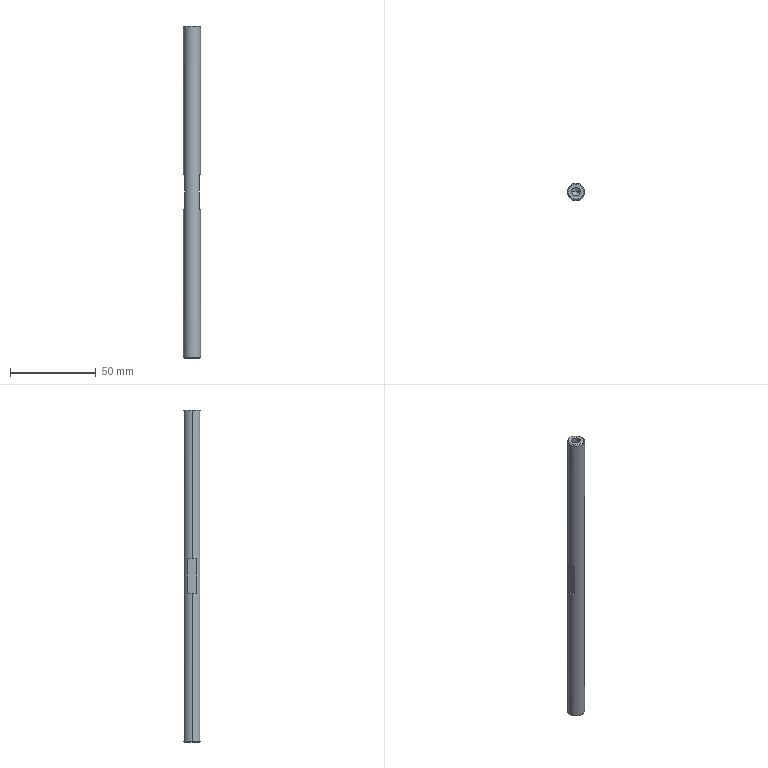Part | SolidWorks | features HoleWzd 2, Chamfer 1, Extrusion 1, ICE 1 | 1 solid | 22 faces | box 10 x 10 x 194 mm | volume 14513 mm3 | cone 8 | plane 8 | cylinder 6 | commonest cylinder face diameters 5 x4 10 x2
STEP:
#1=CARTESIAN_POINT('',(-4.5,0.,-97.));
#2=VERTEX_POINT('',#1);
#3=CARTESIAN_POINT('',(4.5,0.,-97.));
#4=VERTEX_POINT('',#3);
#5=CARTESIAN_POINT('',(0.,0.,-97.));
#6=DIRECTION('',(0.,0.,-1.));
#7=DIRECTION('',(1.,0.,0.));
#8=AXIS2_PLACEMENT_3D('',#5,#6,#7);
#9=CIRCLE('',#8,4.5);
#10=EDGE_CURVE('',#2,#4,#9,.T.);
#11=ORIENTED_EDGE('',*,*,#10,.F.);
#12=CARTESIAN_POINT('',(-5.,0.,-96.5));
#13=VERTEX_POINT('',#12);
#14=CARTESIAN_POINT('',(-5.,0.,-96.5));
#15=DIRECTION('',(-0.7071,0.,0.7071));
#16=VECTOR('',#15,1000.);
#17=LINE('',#14,#16);
#18=EDGE_CURVE('',#2,#13,#17,.T.);
#19=ORIENTED_EDGE('',*,*,#18,.T.);
#20=CARTESIAN_POINT('',(5.,0.,-96.5));
#21=VERTEX_POINT('',#20);
#22=CARTESIAN_POINT('',(0.,0.,-96.5));
#23=DIRECTION('',(0.,0.,1.));
#24=DIRECTION('',(1.,0.,0.));
#25=AXIS2_PLACEMENT_3D('',#22,#23,#24);
#26=CIRCLE('',#25,5.);
#27=EDGE_CURVE('',#21,#13,#26,.T.);
#28=ORIENTED_EDGE('',*,*,#27,.F.);
#29=CARTESIAN_POINT('',(5.,0.,-96.5));
#30=DIRECTION('',(0.7071,0.,0.7071));
#31=VECTOR('',#30,1000.);
#32=LINE('',#29,#31);
#33=EDGE_CURVE('',#4,#21,#32,.T.);
#34=ORIENTED_EDGE('',*,*,#33,.F.);
#35=EDGE_LOOP('',(#11,#19,#28,#34));
#36=FACE_OUTER_BOUND('',#35,.T.);
#37=CARTESIAN_POINT('',(0.,0.,-96.5));
#38=DIRECTION('',(0.,0.,1.));
#39=DIRECTION('',(1.,0.,0.));
#40=AXIS2_PLACEMENT_3D('',#37,#38,#39);
#41=CONICAL_SURFACE('',#40,5.,0.7854);
#42=ADVANCED_FACE('',(#36),#41,.T.);
#43=CARTESIAN_POINT('',(4.5,0.,97.));
#44=VERTEX_POINT('',#43);
#45=CARTESIAN_POINT('',(-4.5,0.,97.));
#46=VERTEX_POINT('',#45);
#47=CARTESIAN_POINT('',(0.,0.,97.));
#48=DIRECTION('',(0.,0.,1.));
#49=DIRECTION('',(1.,0.,0.));
#50=AXIS2_PLACEMENT_3D('',#47,#48,#49);
#51=CIRCLE('',#50,4.5);
#52=EDGE_CURVE('',#44,#46,#51,.T.);
#53=ORIENTED_EDGE('',*,*,#52,.F.);
#54=CARTESIAN_POINT('',(5.,0.,96.5));
#55=VERTEX_POINT('',#54);
#56=CARTESIAN_POINT('',(4.5,0.,97.));
#57=DIRECTION('',(0.7071,0.,-0.7071));
#58=VECTOR('',#57,1000.);
#59=LINE('',#56,#58);
#60=EDGE_CURVE('',#44,#55,#59,.T.);
#61=ORIENTED_EDGE('',*,*,#60,.T.);
#62=CARTESIAN_POINT('',(-5.,0.,96.5));
#63=VERTEX_POINT('',#62);
#64=CARTESIAN_POINT('',(0.,0.,96.5));
#65=DIRECTION('',(0.,0.,-1.));
#66=DIRECTION('',(1.,0.,0.));
#67=AXIS2_PLACEMENT_3D('',#64,#65,#66);
#68=CIRCLE('',#67,5.);
#69=EDGE_CURVE('',#63,#55,#68,.T.);
#70=ORIENTED_EDGE('',*,*,#69,.F.);
#71=CARTESIAN_POINT('',(-4.5,0.,97.));
#72=DIRECTION('',(-0.7071,0.,-0.7071));
#73=VECTOR('',#72,1000.);
#74=LINE('',#71,#73);
#75=EDGE_CURVE('',#46,#63,#74,.T.);
#76=ORIENTED_EDGE('',*,*,#75,.F.);
#77=EDGE_LOOP('',(#53,#61,#70,#76));
#78=FACE_OUTER_BOUND('',#77,.T.);
#79=CARTESIAN_POINT('',(0.,0.,97.));
#80=DIRECTION('',(0.,0.,-1.));
#81=DIRECTION('',(-1.,0.,0.));
#82=AXIS2_PLACEMENT_3D('',#79,#80,#81);
#83=CONICAL_SURFACE('',#82,4.5,0.7854);
#84=ADVANCED_FACE('',(#78),#83,.T.);
#85=CARTESIAN_POINT('',(2.5,0.,-82.));
#86=VERTEX_POINT('',#85);
#87=CARTESIAN_POINT('',(-2.5,0.,-82.));
#88=VERTEX_POINT('',#87);
#89=CARTESIAN_POINT('',(0.,0.,-82.));
#90=DIRECTION('',(0.,0.,-1.));
#91=DIRECTION('',(-1.,0.,0.));
#92=AXIS2_PLACEMENT_3D('',#89,#90,#91);
#93=CIRCLE('',#92,2.5);
#94=EDGE_CURVE('',#86,#88,#93,.T.);
#95=ORIENTED_EDGE('',*,*,#94,.F.);
#96=CARTESIAN_POINT('',(2.5,0.,-97.));
#97=VERTEX_POINT('',#96);
#98=CARTESIAN_POINT('',(2.5,0.,-97.));
#99=DIRECTION('',(0.,0.,-1.));
#100=VECTOR('',#99,1000.);
#101=LINE('',#98,#100);
#102=EDGE_CURVE('',#86,#97,#101,.T.);
#103=ORIENTED_EDGE('',*,*,#102,.T.);
#104=CARTESIAN_POINT('',(-2.5,0.,-97.));
#105=VERTEX_POINT('',#104);
#106=CARTESIAN_POINT('',(0.,0.,-97.));
#107=DIRECTION('',(0.,0.,-1.));
#108=DIRECTION('',(-1.,0.,0.));
#109=AXIS2_PLACEMENT_3D('',#106,#107,#108);
#110=CIRCLE('',#109,2.5);
#111=EDGE_CURVE('',#97,#105,#110,.T.);
#112=ORIENTED_EDGE('',*,*,#111,.T.);
#113=CARTESIAN_POINT('',(-2.5,0.,-97.));
#114=DIRECTION('',(0.,0.,-1.));
#115=VECTOR('',#114,1000.);
#116=LINE('',#113,#115);
#117=EDGE_CURVE('',#88,#105,#116,.T.);
#118=ORIENTED_EDGE('',*,*,#117,.F.);
#119=EDGE_LOOP('',(#95,#103,#112,#118));
#120=FACE_OUTER_BOUND('',#119,.T.);
#121=CARTESIAN_POINT('',(0.,0.,-97.));
#122=DIRECTION('',(0.,0.,-1.));
#123=DIRECTION('',(-1.,0.,0.));
#124=AXIS2_PLACEMENT_3D('',#121,#122,#123);
#125=CYLINDRICAL_SURFACE('',#124,2.5);
#126=ADVANCED_FACE('',(#120),#125,.F.);
#127=CARTESIAN_POINT('',(0.,0.,-80.498));
#128=VERTEX_POINT('',#127);
#129=CARTESIAN_POINT('',(-2.5,0.,-82.));
#130=DIRECTION('',(-0.8572,0.,-0.515));
#131=VECTOR('',#130,1000.);
#132=LINE('',#129,#131);
#133=EDGE_CURVE('',#128,#88,#132,.T.);
#134=ORIENTED_EDGE('',*,*,#133,.F.);
#135=CARTESIAN_POINT('',(2.5,0.,-82.));
#136=DIRECTION('',(0.8572,0.,-0.515));
#137=VECTOR('',#136,1000.);
#138=LINE('',#135,#137);
#139=EDGE_CURVE('',#128,#86,#138,.T.);
#140=ORIENTED_EDGE('',*,*,#139,.T.);
#141=ORIENTED_EDGE('',*,*,#94,.T.);
#142=EDGE_LOOP('',(#134,#140,#141));
#143=FACE_OUTER_BOUND('',#142,.T.);
#144=CARTESIAN_POINT('',(0.,0.,-82.));
#145=DIRECTION('',(0.,0.,-1.));
#146=DIRECTION('',(-1.,0.,0.));
#147=AXIS2_PLACEMENT_3D('',#144,#145,#146);
#148=CONICAL_SURFACE('',#147,2.5,1.03);
#149=ADVANCED_FACE('',(#143),#148,.F.);
#150=CARTESIAN_POINT('',(-2.5,0.,82.));
#151=VERTEX_POINT('',#150);
#152=CARTESIAN_POINT('',(2.5,0.,82.));
#153=VERTEX_POINT('',#152);
#154=CARTESIAN_POINT('',(0.,0.,82.));
#155=DIRECTION('',(0.,0.,1.));
#156=DIRECTION('',(1.,0.,0.));
#157=AXIS2_PLACEMENT_3D('',#154,#155,#156);
#158=CIRCLE('',#157,2.5);
#159=EDGE_CURVE('',#151,#153,#158,.T.);
#160=ORIENTED_EDGE('',*,*,#159,.F.);
#161=CARTESIAN_POINT('',(-2.5,0.,97.));
#162=VERTEX_POINT('',#161);
#163=CARTESIAN_POINT('',(-2.5,0.,97.));
#164=DIRECTION('',(0.,0.,1.));
#165=VECTOR('',#164,1000.);
#166=LINE('',#163,#165);
#167=EDGE_CURVE('',#151,#162,#166,.T.);
#168=ORIENTED_EDGE('',*,*,#167,.T.);
#169=CARTESIAN_POINT('',(2.5,0.,97.));
#170=VERTEX_POINT('',#169);
#171=CARTESIAN_POINT('',(0.,0.,97.));
#172=DIRECTION('',(0.,0.,1.));
#173=DIRECTION('',(1.,0.,0.));
#174=AXIS2_PLACEMENT_3D('',#171,#172,#173);
#175=CIRCLE('',#174,2.5);
#176=EDGE_CURVE('',#162,#170,#175,.T.);
#177=ORIENTED_EDGE('',*,*,#176,.T.);
#178=CARTESIAN_POINT('',(2.5,0.,97.));
#179=DIRECTION('',(0.,0.,1.));
#180=VECTOR('',#179,1000.);
#181=LINE('',#178,#180);
#182=EDGE_CURVE('',#153,#170,#181,.T.);
#183=ORIENTED_EDGE('',*,*,#182,.F.);
#184=EDGE_LOOP('',(#160,#168,#177,#183));
#185=FACE_OUTER_BOUND('',#184,.T.);
#186=CARTESIAN_POINT('',(0.,0.,97.));
#187=DIRECTION('',(0.,0.,1.));
#188=DIRECTION('',(1.,0.,0.));
#189=AXIS2_PLACEMENT_3D('',#186,#187,#188);
#190=CYLINDRICAL_SURFACE('',#189,2.5);
#191=ADVANCED_FACE('',(#185),#190,.F.);
#192=CARTESIAN_POINT('',(0.,0.,80.498));
#193=VERTEX_POINT('',#192);
#194=CARTESIAN_POINT('',(2.5,0.,82.));
#195=DIRECTION('',(0.8572,0.,0.515));
#196=VECTOR('',#195,1000.);
#197=LINE('',#194,#196);
#198=EDGE_CURVE('',#193,#153,#197,.T.);
#199=ORIENTED_EDGE('',*,*,#198,.F.);
#200=CARTESIAN_POINT('',(-2.5,0.,82.));
#201=DIRECTION('',(-0.8572,0.,0.515));
#202=VECTOR('',#201,1000.);
#203=LINE('',#200,#202);
#204=EDGE_CURVE('',#193,#151,#203,.T.);
#205=ORIENTED_EDGE('',*,*,#204,.T.);
#206=ORIENTED_EDGE('',*,*,#159,.T.);
#207=EDGE_LOOP('',(#199,#205,#206));
#208=FACE_OUTER_BOUND('',#207,.T.);
#209=CARTESIAN_POINT('',(0.,0.,82.));
#210=DIRECTION('',(0.,0.,1.));
#211=DIRECTION('',(1.,0.,0.));
#212=AXIS2_PLACEMENT_3D('',#209,#210,#211);
#213=CONICAL_SURFACE('',#212,2.5,1.03);
#214=ADVANCED_FACE('',(#208),#213,.F.);
#215=ORIENTED_EDGE('',*,*,#69,.T.);
#216=CARTESIAN_POINT('',(5.,0.,10.));
#217=VERTEX_POINT('',#216);
#218=CARTESIAN_POINT('',(5.,0.,97.));
#219=DIRECTION('',(0.,0.,-1.));
#220=VECTOR('',#219,1000.);
#221=LINE('',#218,#220);
#222=EDGE_CURVE('',#55,#217,#221,.T.);
#223=ORIENTED_EDGE('',*,*,#222,.T.);
#224=CARTESIAN_POINT('',(4.25,2.634,10.));
#225=VERTEX_POINT('',#224);
#226=CARTESIAN_POINT('',(0.,0.,10.));
#227=DIRECTION('',(0.,0.,1.));
#228=DIRECTION('',(1.,0.,0.));
#229=AXIS2_PLACEMENT_3D('',#226,#227,#228);
#230=CIRCLE('',#229,5.);
#231=EDGE_CURVE('',#217,#225,#230,.T.);
#232=ORIENTED_EDGE('',*,*,#231,.T.);
#233=CARTESIAN_POINT('',(4.25,2.634,-10.));
#234=VERTEX_POINT('',#233);
#235=CARTESIAN_POINT('',(4.25,2.634,-10.));
#236=DIRECTION('',(0.,0.,1.));
#237=VECTOR('',#236,1000.);
#238=LINE('',#235,#237);
#239=EDGE_CURVE('',#234,#225,#238,.T.);
#240=ORIENTED_EDGE('',*,*,#239,.F.);
#241=CARTESIAN_POINT('',(5.,0.,-10.));
#242=VERTEX_POINT('',#241);
#243=CARTESIAN_POINT('',(0.,0.,-10.));
#244=DIRECTION('',(0.,0.,1.));
#245=DIRECTION('',(1.,0.,0.));
#246=AXIS2_PLACEMENT_3D('',#243,#244,#245);
#247=CIRCLE('',#246,5.);
#248=EDGE_CURVE('',#242,#234,#247,.T.);
#249=ORIENTED_EDGE('',*,*,#248,.F.);
#250=CARTESIAN_POINT('',(5.,0.,97.));
#251=DIRECTION('',(0.,0.,-1.));
#252=VECTOR('',#251,1000.);
#253=LINE('',#250,#252);
#254=EDGE_CURVE('',#242,#21,#253,.T.);
#255=ORIENTED_EDGE('',*,*,#254,.T.);
#256=ORIENTED_EDGE('',*,*,#27,.T.);
#257=CARTESIAN_POINT('',(-5.,0.,-10.));
#258=VERTEX_POINT('',#257);
#259=CARTESIAN_POINT('',(-5.,0.,97.));
#260=DIRECTION('',(0.,0.,-1.));
#261=VECTOR('',#260,1000.);
#262=LINE('',#259,#261);
#263=EDGE_CURVE('',#258,#13,#262,.T.);
#264=ORIENTED_EDGE('',*,*,#263,.F.);
#265=CARTESIAN_POINT('',(-4.25,2.634,-10.));
#266=VERTEX_POINT('',#265);
#267=CARTESIAN_POINT('',(0.,0.,-10.));
#268=DIRECTION('',(0.,0.,1.));
#269=DIRECTION('',(1.,0.,0.));
#270=AXIS2_PLACEMENT_3D('',#267,#268,#269);
#271=CIRCLE('',#270,5.);
#272=EDGE_CURVE('',#266,#258,#271,.T.);
#273=ORIENTED_EDGE('',*,*,#272,.F.);
#274=CARTESIAN_POINT('',(-4.25,2.634,10.));
#275=VERTEX_POINT('',#274);
#276=CARTESIAN_POINT('',(-4.25,2.634,-10.));
#277=DIRECTION('',(0.,0.,1.));
#278=VECTOR('',#277,1000.);
#279=LINE('',#276,#278);
#280=EDGE_CURVE('',#266,#275,#279,.T.);
#281=ORIENTED_EDGE('',*,*,#280,.T.);
#282=CARTESIAN_POINT('',(-5.,0.,10.));
#283=VERTEX_POINT('',#282);
#284=CARTESIAN_POINT('',(0.,0.,10.));
#285=DIRECTION('',(0.,0.,1.));
#286=DIRECTION('',(1.,0.,0.));
#287=AXIS2_PLACEMENT_3D('',#284,#285,#286);
#288=CIRCLE('',#287,5.);
#289=EDGE_CURVE('',#275,#283,#288,.T.);
#290=ORIENTED_EDGE('',*,*,#289,.T.);
#291=CARTESIAN_POINT('',(-5.,0.,97.));
#292=DIRECTION('',(0.,0.,-1.));
#293=VECTOR('',#292,1000.);
#294=LINE('',#291,#293);
#295=EDGE_CURVE('',#63,#283,#294,.T.);
#296=ORIENTED_EDGE('',*,*,#295,.F.);
#297=EDGE_LOOP('',(#215,#223,#232,#240,#249,#255,#256,#264,#273,#281,#290,#296));
#298=FACE_OUTER_BOUND('',#297,.T.);
#299=CARTESIAN_POINT('',(0.,0.,97.));
#300=DIRECTION('',(0.,0.,-1.));
#301=DIRECTION('',(-1.,0.,0.));
#302=AXIS2_PLACEMENT_3D('',#299,#300,#301);
#303=CYLINDRICAL_SURFACE('',#302,5.);
#304=ADVANCED_FACE('',(#298),#303,.T.);
#305=ORIENTED_EDGE('',*,*,#222,.F.);
#306=CARTESIAN_POINT('',(0.,0.,96.5));
#307=DIRECTION('',(0.,0.,-1.));
#308=DIRECTION('',(1.,0.,0.));
#309=AXIS2_PLACEMENT_3D('',#306,#307,#308);
#310=CIRCLE('',#309,5.);
#311=EDGE_CURVE('',#55,#63,#310,.T.);
#312=ORIENTED_EDGE('',*,*,#311,.T.);
#313=ORIENTED_EDGE('',*,*,#295,.T.);
#314=CARTESIAN_POINT('',(-4.25,-2.634,10.));
#315=VERTEX_POINT('',#314);
#316=CARTESIAN_POINT('',(0.,0.,10.));
#317=DIRECTION('',(0.,0.,1.));
#318=DIRECTION('',(1.,0.,0.));
#319=AXIS2_PLACEMENT_3D('',#316,#317,#318);
#320=CIRCLE('',#319,5.);
#321=EDGE_CURVE('',#283,#315,#320,.T.);
#322=ORIENTED_EDGE('',*,*,#321,.T.);
#323=CARTESIAN_POINT('',(-4.25,-2.634,-10.));
#324=VERTEX_POINT('',#323);
#325=CARTESIAN_POINT('',(-4.25,-2.634,-10.));
#326=DIRECTION('',(0.,0.,1.));
#327=VECTOR('',#326,1000.);
#328=LINE('',#325,#327);
#329=EDGE_CURVE('',#324,#315,#328,.T.);
#330=ORIENTED_EDGE('',*,*,#329,.F.);
#331=CARTESIAN_POINT('',(0.,0.,-10.));
#332=DIRECTION('',(0.,0.,1.));
#333=DIRECTION('',(1.,0.,0.));
#334=AXIS2_PLACEMENT_3D('',#331,#332,#333);
#335=CIRCLE('',#334,5.);
#336=EDGE_CURVE('',#258,#324,#335,.T.);
#337=ORIENTED_EDGE('',*,*,#336,.F.);
#338=ORIENTED_EDGE('',*,*,#263,.T.);
#339=CARTESIAN_POINT('',(0.,0.,-96.5));
#340=DIRECTION('',(0.,0.,1.));
#341=DIRECTION('',(1.,0.,0.));
#342=AXIS2_PLACEMENT_3D('',#339,#340,#341);
#343=CIRCLE('',#342,5.);
#344=EDGE_CURVE('',#13,#21,#343,.T.);
#345=ORIENTED_EDGE('',*,*,#344,.T.);
#346=ORIENTED_EDGE('',*,*,#254,.F.);
#347=CARTESIAN_POINT('',(4.25,-2.634,-10.));
#348=VERTEX_POINT('',#347);
#349=CARTESIAN_POINT('',(0.,0.,-10.));
#350=DIRECTION('',(0.,0.,1.));
#351=DIRECTION('',(1.,0.,0.));
#352=AXIS2_PLACEMENT_3D('',#349,#350,#351);
#353=CIRCLE('',#352,5.);
#354=EDGE_CURVE('',#348,#242,#353,.T.);
#355=ORIENTED_EDGE('',*,*,#354,.F.);
#356=CARTESIAN_POINT('',(4.25,-2.634,10.));
#357=VERTEX_POINT('',#356);
#358=CARTESIAN_POINT('',(4.25,-2.634,-10.));
#359=DIRECTION('',(0.,0.,1.));
#360=VECTOR('',#359,1000.);
#361=LINE('',#358,#360);
#362=EDGE_CURVE('',#348,#357,#361,.T.);
#363=ORIENTED_EDGE('',*,*,#362,.T.);
#364=CARTESIAN_POINT('',(0.,0.,10.));
#365=DIRECTION('',(0.,0.,1.));
#366=DIRECTION('',(1.,0.,0.));
#367=AXIS2_PLACEMENT_3D('',#364,#365,#366);
#368=CIRCLE('',#367,5.);
#369=EDGE_CURVE('',#357,#217,#368,.T.);
#370=ORIENTED_EDGE('',*,*,#369,.T.);
#371=EDGE_LOOP('',(#305,#312,#313,#322,#330,#337,#338,#345,#346,#355,#363,#370));
#372=FACE_OUTER_BOUND('',#371,.T.);
#373=CARTESIAN_POINT('',(0.,0.,97.));
#374=DIRECTION('',(0.,0.,-1.));
#375=DIRECTION('',(-1.,0.,0.));
#376=AXIS2_PLACEMENT_3D('',#373,#374,#375);
#377=CYLINDRICAL_SURFACE('',#376,5.);
#378=ADVANCED_FACE('',(#372),#377,.T.);
#379=CARTESIAN_POINT('',(0.,0.,97.));
#380=DIRECTION('',(0.,0.,1.));
#381=DIRECTION('',(1.,0.,0.));
#382=AXIS2_PLACEMENT_3D('',#379,#380,#381);
#383=CIRCLE('',#382,4.5);
#384=EDGE_CURVE('',#46,#44,#383,.T.);
#385=ORIENTED_EDGE('',*,*,#384,.T.);
#386=ORIENTED_EDGE('',*,*,#52,.T.);
#387=EDGE_LOOP('',(#385,#386));
#388=FACE_OUTER_BOUND('',#387,.T.);
#389=CARTESIAN_POINT('',(0.,0.,97.));
#390=DIRECTION('',(0.,0.,1.));
#391=DIRECTION('',(1.,0.,0.));
#392=AXIS2_PLACEMENT_3D('',#389,#390,#391);
#393=CIRCLE('',#392,2.5);
#394=EDGE_CURVE('',#170,#162,#393,.T.);
#395=ORIENTED_EDGE('',*,*,#394,.F.);
#396=ORIENTED_EDGE('',*,*,#176,.F.);
#397=EDGE_LOOP('',(#395,#396));
#398=FACE_BOUND('',#397,.T.);
#399=CARTESIAN_POINT('',(0.,0.,97.));
#400=DIRECTION('',(0.,0.,1.));
#401=DIRECTION('',(1.,0.,0.));
#402=AXIS2_PLACEMENT_3D('',#399,#400,#401);
#403=PLANE('',#402);
#404=ADVANCED_FACE('',(#388,#398),#403,.T.);
#405=CARTESIAN_POINT('',(0.,0.,-97.));
#406=DIRECTION('',(0.,0.,-1.));
#407=DIRECTION('',(1.,0.,0.));
#408=AXIS2_PLACEMENT_3D('',#405,#406,#407);
#409=CIRCLE('',#408,4.5);
#410=EDGE_CURVE('',#4,#2,#409,.T.);
#411=ORIENTED_EDGE('',*,*,#410,.T.);
#412=ORIENTED_EDGE('',*,*,#10,.T.);
#413=EDGE_LOOP('',(#411,#412));
#414=FACE_OUTER_BOUND('',#413,.T.);
#415=CARTESIAN_POINT('',(0.,0.,-97.));
#416=DIRECTION('',(0.,0.,-1.));
#417=DIRECTION('',(-1.,0.,0.));
#418=AXIS2_PLACEMENT_3D('',#415,#416,#417);
#419=CIRCLE('',#418,2.5);
#420=EDGE_CURVE('',#105,#97,#419,.T.);
#421=ORIENTED_EDGE('',*,*,#420,.F.);
#422=ORIENTED_EDGE('',*,*,#111,.F.);
#423=EDGE_LOOP('',(#421,#422));
#424=FACE_BOUND('',#423,.T.);
#425=CARTESIAN_POINT('',(0.,0.,-97.));
#426=DIRECTION('',(0.,0.,1.));
#427=DIRECTION('',(1.,0.,0.));
#428=AXIS2_PLACEMENT_3D('',#425,#426,#427);
#429=PLANE('',#428);
#430=ADVANCED_FACE('',(#414,#424),#429,.F.);
#431=CARTESIAN_POINT('',(4.25,2.634,10.));
#432=DIRECTION('',(0.,-1.,0.));
#433=VECTOR('',#432,1000.);
#434=LINE('',#431,#433);
#435=EDGE_CURVE('',#225,#357,#434,.T.);
#436=ORIENTED_EDGE('',*,*,#435,.T.);
#437=ORIENTED_EDGE('',*,*,#362,.F.);
#438=CARTESIAN_POINT('',(4.25,2.634,-10.));
#439=DIRECTION('',(0.,-1.,0.));
#440=VECTOR('',#439,1000.);
#441=LINE('',#438,#440);
#442=EDGE_CURVE('',#234,#348,#441,.T.);
#443=ORIENTED_EDGE('',*,*,#442,.F.);
#444=ORIENTED_EDGE('',*,*,#239,.T.);
#445=EDGE_LOOP('',(#436,#437,#443,#444));
#446=FACE_OUTER_BOUND('',#445,.T.);
#447=CARTESIAN_POINT('',(4.25,2.634,-10.));
#448=DIRECTION('',(-1.,0.,0.));
#449=DIRECTION('',(0.,0.,1.));
#450=AXIS2_PLACEMENT_3D('',#447,#448,#449);
#451=PLANE('',#450);
#452=ADVANCED_FACE('',(#446),#451,.F.);
#453=ORIENTED_EDGE('',*,*,#354,.T.);
#454=ORIENTED_EDGE('',*,*,#248,.T.);
#455=ORIENTED_EDGE('',*,*,#442,.T.);
#456=EDGE_LOOP('',(#453,#454,#455));
#457=FACE_OUTER_BOUND('',#456,.T.);
#458=CARTESIAN_POINT('',(0.,0.,-10.));
#459=DIRECTION('',(0.,0.,1.));
#460=DIRECTION('',(1.,0.,0.));
#461=AXIS2_PLACEMENT_3D('',#458,#459,#460);
#462=PLANE('',#461);
#463=ADVANCED_FACE('',(#457),#462,.T.);
#464=ORIENTED_EDGE('',*,*,#369,.F.);
#465=ORIENTED_EDGE('',*,*,#435,.F.);
#466=ORIENTED_EDGE('',*,*,#231,.F.);
#467=EDGE_LOOP('',(#464,#465,#466));
#468=FACE_OUTER_BOUND('',#467,.T.);
#469=CARTESIAN_POINT('',(0.,0.,10.));
#470=DIRECTION('',(0.,0.,1.));
#471=DIRECTION('',(1.,0.,0.));
#472=AXIS2_PLACEMENT_3D('',#469,#470,#471);
#473=PLANE('',#472);
#474=ADVANCED_FACE('',(#468),#473,.F.);
#475=CARTESIAN_POINT('',(-4.25,2.634,10.));
#476=DIRECTION('',(0.,1.,0.));
#477=VECTOR('',#476,1000.);
#478=LINE('',#475,#477);
#479=EDGE_CURVE('',#315,#275,#478,.T.);
#480=ORIENTED_EDGE('',*,*,#479,.T.);
#481=ORIENTED_EDGE('',*,*,#280,.F.);
#482=CARTESIAN_POINT('',(-4.25,2.634,-10.));
#483=DIRECTION('',(0.,1.,0.));
#484=VECTOR('',#483,1000.);
#485=LINE('',#482,#484);
#486=EDGE_CURVE('',#324,#266,#485,.T.);
#487=ORIENTED_EDGE('',*,*,#486,.F.);
#488=ORIENTED_EDGE('',*,*,#329,.T.);
#489=EDGE_LOOP('',(#480,#481,#487,#488));
#490=FACE_OUTER_BOUND('',#489,.T.);
#491=CARTESIAN_POINT('',(-4.25,2.634,-10.));
#492=DIRECTION('',(1.,0.,0.));
#493=DIRECTION('',(0.,0.,-1.));
#494=AXIS2_PLACEMENT_3D('',#491,#492,#493);
#495=PLANE('',#494);
#496=ADVANCED_FACE('',(#490),#495,.F.);
#497=ORIENTED_EDGE('',*,*,#272,.T.);
#498=ORIENTED_EDGE('',*,*,#336,.T.);
#499=ORIENTED_EDGE('',*,*,#486,.T.);
#500=EDGE_LOOP('',(#497,#498,#499));
#501=FACE_OUTER_BOUND('',#500,.T.);
#502=CARTESIAN_POINT('',(0.,0.,-10.));
#503=DIRECTION('',(0.,0.,1.));
#504=DIRECTION('',(1.,0.,0.));
#505=AXIS2_PLACEMENT_3D('',#502,#503,#504);
#506=PLANE('',#505);
#507=ADVANCED_FACE('',(#501),#506,.T.);
#508=ORIENTED_EDGE('',*,*,#289,.F.);
#509=ORIENTED_EDGE('',*,*,#479,.F.);
#510=ORIENTED_EDGE('',*,*,#321,.F.);
#511=EDGE_LOOP('',(#508,#509,#510));
#512=FACE_OUTER_BOUND('',#511,.T.);
#513=CARTESIAN_POINT('',(0.,0.,10.));
#514=DIRECTION('',(0.,0.,1.));
#515=DIRECTION('',(1.,0.,0.));
#516=AXIS2_PLACEMENT_3D('',#513,#514,#515);
#517=PLANE('',#516);
#518=ADVANCED_FACE('',(#512),#517,.F.);
#519=ORIENTED_EDGE('',*,*,#204,.F.);
#520=ORIENTED_EDGE('',*,*,#198,.T.);
#521=CARTESIAN_POINT('',(0.,0.,82.));
#522=DIRECTION('',(0.,0.,1.));
#523=DIRECTION('',(1.,0.,0.));
#524=AXIS2_PLACEMENT_3D('',#521,#522,#523);
#525=CIRCLE('',#524,2.5);
#526=EDGE_CURVE('',#153,#151,#525,.T.);
#527=ORIENTED_EDGE('',*,*,#526,.T.);
#528=EDGE_LOOP('',(#519,#520,#527));
#529=FACE_OUTER_BOUND('',#528,.T.);
#530=CARTESIAN_POINT('',(0.,0.,82.));
#531=DIRECTION('',(0.,0.,1.));
#532=DIRECTION('',(1.,0.,0.));
#533=AXIS2_PLACEMENT_3D('',#530,#531,#532);
#534=CONICAL_SURFACE('',#533,2.5,1.03);
#535=ADVANCED_FACE('',(#529),#534,.F.);
#536=ORIENTED_EDGE('',*,*,#167,.F.);
#537=ORIENTED_EDGE('',*,*,#526,.F.);
#538=ORIENTED_EDGE('',*,*,#182,.T.);
#539=ORIENTED_EDGE('',*,*,#394,.T.);
#540=EDGE_LOOP('',(#536,#537,#538,#539));
#541=FACE_OUTER_BOUND('',#540,.T.);
#542=CARTESIAN_POINT('',(0.,0.,97.));
#543=DIRECTION('',(0.,0.,1.));
#544=DIRECTION('',(1.,0.,0.));
#545=AXIS2_PLACEMENT_3D('',#542,#543,#544);
#546=CYLINDRICAL_SURFACE('',#545,2.5);
#547=ADVANCED_FACE('',(#541),#546,.F.);
#548=ORIENTED_EDGE('',*,*,#139,.F.);
#549=ORIENTED_EDGE('',*,*,#133,.T.);
#550=CARTESIAN_POINT('',(0.,0.,-82.));
#551=DIRECTION('',(0.,0.,-1.));
#552=DIRECTION('',(-1.,0.,0.));
#553=AXIS2_PLACEMENT_3D('',#550,#551,#552);
#554=CIRCLE('',#553,2.5);
#555=EDGE_CURVE('',#88,#86,#554,.T.);
#556=ORIENTED_EDGE('',*,*,#555,.T.);
#557=EDGE_LOOP('',(#548,#549,#556));
#558=FACE_OUTER_BOUND('',#557,.T.);
#559=CARTESIAN_POINT('',(0.,0.,-82.));
#560=DIRECTION('',(0.,0.,-1.));
#561=DIRECTION('',(-1.,0.,0.));
#562=AXIS2_PLACEMENT_3D('',#559,#560,#561);
#563=CONICAL_SURFACE('',#562,2.5,1.03);
#564=ADVANCED_FACE('',(#558),#563,.F.);
#565=ORIENTED_EDGE('',*,*,#102,.F.);
#566=ORIENTED_EDGE('',*,*,#555,.F.);
#567=ORIENTED_EDGE('',*,*,#117,.T.);
#568=ORIENTED_EDGE('',*,*,#420,.T.);
#569=EDGE_LOOP('',(#565,#566,#567,#568));
#570=FACE_OUTER_BOUND('',#569,.T.);
#571=CARTESIAN_POINT('',(0.,0.,-97.));
#572=DIRECTION('',(0.,0.,-1.));
#573=DIRECTION('',(-1.,0.,0.));
#574=AXIS2_PLACEMENT_3D('',#571,#572,#573);
#575=CYLINDRICAL_SURFACE('',#574,2.5);
#576=ADVANCED_FACE('',(#570),#575,.F.);
#577=ORIENTED_EDGE('',*,*,#60,.F.);
#578=ORIENTED_EDGE('',*,*,#384,.F.);
#579=ORIENTED_EDGE('',*,*,#75,.T.);
#580=ORIENTED_EDGE('',*,*,#311,.F.);
#581=EDGE_LOOP('',(#577,#578,#579,#580));
#582=FACE_OUTER_BOUND('',#581,.T.);
#583=CARTESIAN_POINT('',(0.,0.,97.));
#584=DIRECTION('',(0.,0.,-1.));
#585=DIRECTION('',(-1.,0.,0.));
#586=AXIS2_PLACEMENT_3D('',#583,#584,#585);
#587=CONICAL_SURFACE('',#586,4.5,0.7854);
#588=ADVANCED_FACE('',(#582),#587,.T.);
#589=ORIENTED_EDGE('',*,*,#18,.F.);
#590=ORIENTED_EDGE('',*,*,#410,.F.);
#591=ORIENTED_EDGE('',*,*,#33,.T.);
#592=ORIENTED_EDGE('',*,*,#344,.F.);
#593=EDGE_LOOP('',(#589,#590,#591,#592));
#594=FACE_OUTER_BOUND('',#593,.T.);
#595=CARTESIAN_POINT('',(0.,0.,-96.5));
#596=DIRECTION('',(0.,0.,1.));
#597=DIRECTION('',(1.,0.,0.));
#598=AXIS2_PLACEMENT_3D('',#595,#596,#597);
#599=CONICAL_SURFACE('',#598,5.,0.7854);
#600=ADVANCED_FACE('',(#594),#599,.T.);
#601=CLOSED_SHELL('',(#42,#84,#126,#149,#191,#214,#304,#378,#404,#430,#452,#463,#474,#496,#507,#518,#535,#547,#564,#576,#588,#600));
#602=MANIFOLD_SOLID_BREP('',#601);
#603=CARTESIAN_POINT('',(0.,0.,0.));
#604=DIRECTION('',(0.,0.,1.));
#605=DIRECTION('',(1.,0.,0.));
#606=AXIS2_PLACEMENT_3D('',#603,#604,#605);
#607=(LENGTH_UNIT()NAMED_UNIT(*)SI_UNIT(.MILLI.,.METRE.));
#608=UNCERTAINTY_MEASURE_WITH_UNIT(LENGTH_MEASURE(0.00001),#607,'','');
#609=(NAMED_UNIT(*)PLANE_ANGLE_UNIT()SI_UNIT($,.RADIAN.));
#610=(NAMED_UNIT(*)SI_UNIT($,.STERADIAN.)SOLID_ANGLE_UNIT());
#611=(GEOMETRIC_REPRESENTATION_CONTEXT(3)GLOBAL_UNCERTAINTY_ASSIGNED_CONTEXT((#608))GLOBAL_UNIT_ASSIGNED_CONTEXT((#607,#609,#610))REPRESENTATION_CONTEXT('',''));
#612=ADVANCED_BREP_SHAPE_REPRESENTATION('',(#602,#606),#611);